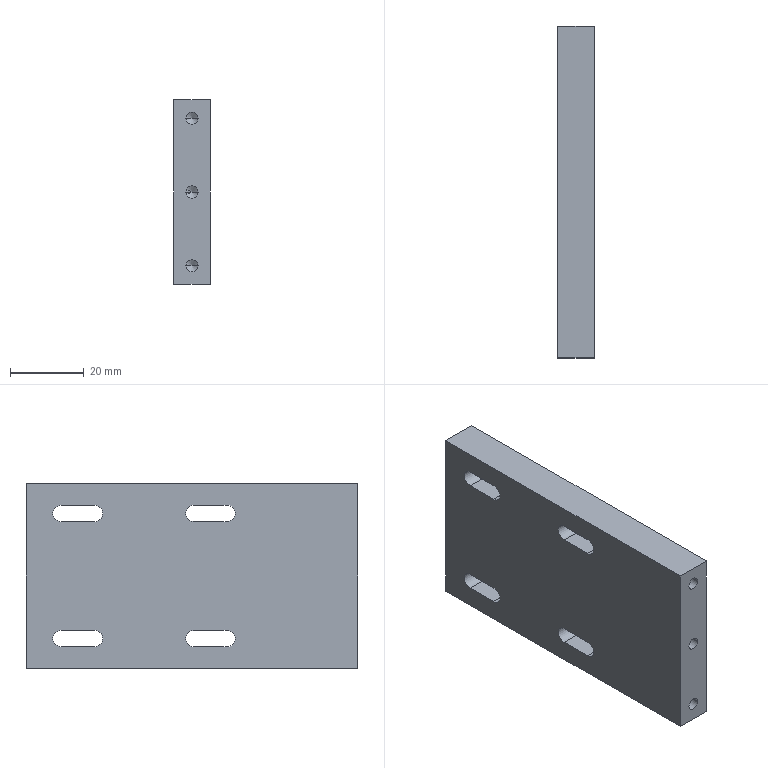Part | STEP file | 04-10 Guide cylinder fixing plate | 1 solid | 34 faces | box 10 x 90 x 50 mm | volume 42374 mm3 | cylinder 14 | plane 14 | cone 6 | commonest cylinder face diameters 4.5 x8 3.3 x6